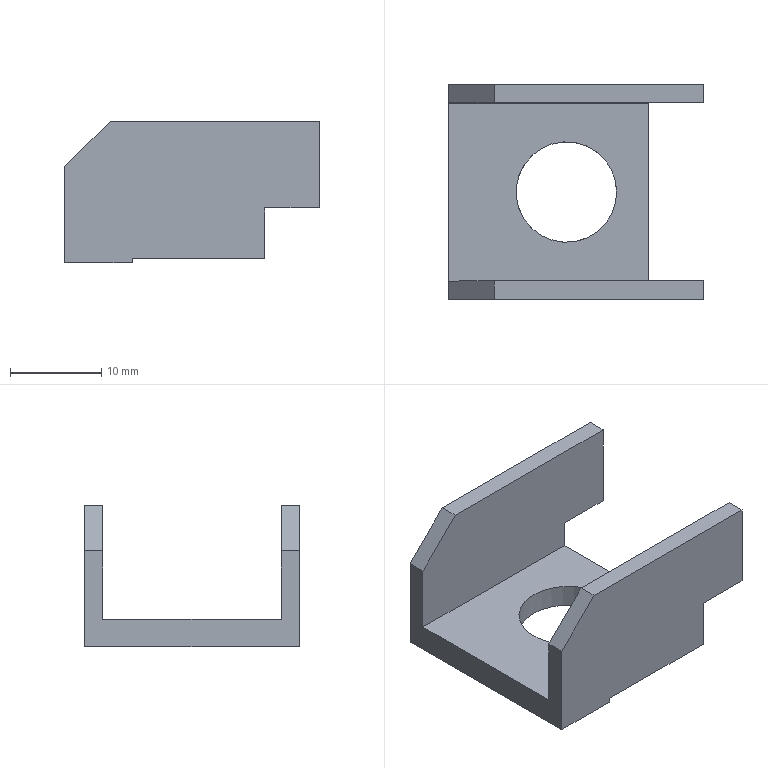Part | NX | features MAIN_BODY 2 | 1 solid | 19 faces | box 27.9 x 23.5 x 15.5 mm | volume 2409 mm3 | plane 18 | cylinder 1 | commonest cylinder face diameters 11 x1
STEP:
#1=CARTESIAN_POINT('',(961.102,239.333,238.));
#2=VERTEX_POINT('',#1);
#3=CARTESIAN_POINT('',(961.102,219.833,238.));
#4=VERTEX_POINT('',#3);
#5=CARTESIAN_POINT('',(961.102,241.333,238.));
#6=DIRECTION('',(0.,-1.,0.));
#7=VECTOR('',#6,1000.);
#8=LINE('',#5,#7);
#9=EDGE_CURVE('',#2,#4,#8,.T.);
#10=ORIENTED_EDGE('',*,*,#9,.T.);
#11=CARTESIAN_POINT('',(983.002,219.833,238.));
#12=VERTEX_POINT('',#11);
#13=CARTESIAN_POINT('',(973.552,219.833,238.));
#14=DIRECTION('',(-1.,0.,0.));
#15=VECTOR('',#14,1000.);
#16=LINE('',#13,#15);
#17=EDGE_CURVE('',#12,#4,#16,.T.);
#18=ORIENTED_EDGE('',*,*,#17,.F.);
#19=CARTESIAN_POINT('',(983.002,239.333,238.));
#20=VERTEX_POINT('',#19);
#21=CARTESIAN_POINT('',(983.002,241.333,238.));
#22=DIRECTION('',(0.,-1.,0.));
#23=VECTOR('',#22,1000.);
#24=LINE('',#21,#23);
#25=EDGE_CURVE('',#20,#12,#24,.T.);
#26=ORIENTED_EDGE('',*,*,#25,.F.);
#27=CARTESIAN_POINT('',(973.552,239.333,238.));
#28=DIRECTION('',(1.,0.,0.));
#29=VECTOR('',#28,1000.);
#30=LINE('',#27,#29);
#31=EDGE_CURVE('',#2,#20,#30,.T.);
#32=ORIENTED_EDGE('',*,*,#31,.F.);
#33=EDGE_LOOP('',(#10,#18,#26,#32));
#34=FACE_BOUND('',#33,.T.);
#35=CARTESIAN_POINT('',(979.502,229.583,238.));
#36=VERTEX_POINT('',#35);
#37=CARTESIAN_POINT('',(974.002,229.583,238.));
#38=DIRECTION('',(0.,0.,1.));
#39=DIRECTION('',(1.,0.,0.));
#40=AXIS2_PLACEMENT_3D('',#37,#38,#39);
#41=CIRCLE('',#40,5.5);
#42=EDGE_CURVE('',#36,#36,#41,.F.);
#43=ORIENTED_EDGE('',*,*,#42,.T.);
#44=EDGE_LOOP('',(#43));
#45=FACE_BOUND('',#44,.T.);
#46=CARTESIAN_POINT('',(973.552,229.583,238.));
#47=DIRECTION('',(0.,0.,-1.));
#48=DIRECTION('',(1.,0.,0.));
#49=AXIS2_PLACEMENT_3D('',#46,#47,#48);
#50=PLANE('',#49);
#51=ADVANCED_FACE('',(#34,#45),#50,.F.);
#52=CARTESIAN_POINT('',(968.502,241.333,235.5));
#53=VERTEX_POINT('',#52);
#54=CARTESIAN_POINT('',(968.502,229.583,235.5));
#55=VERTEX_POINT('',#54);
#56=CARTESIAN_POINT('',(968.502,241.333,235.5));
#57=DIRECTION('',(0.,-1.,0.));
#58=VECTOR('',#57,1000.);
#59=LINE('',#56,#58);
#60=EDGE_CURVE('',#53,#55,#59,.T.);
#61=ORIENTED_EDGE('',*,*,#60,.F.);
#62=CARTESIAN_POINT('',(983.002,241.333,235.5));
#63=VERTEX_POINT('',#62);
#64=CARTESIAN_POINT('',(983.002,241.333,235.5));
#65=DIRECTION('',(1.,0.,0.));
#66=VECTOR('',#65,1000.);
#67=LINE('',#64,#66);
#68=EDGE_CURVE('',#63,#53,#67,.F.);
#69=ORIENTED_EDGE('',*,*,#68,.F.);
#70=CARTESIAN_POINT('',(983.002,217.833,235.5));
#71=VERTEX_POINT('',#70);
#72=CARTESIAN_POINT('',(983.002,241.333,235.5));
#73=DIRECTION('',(0.,1.,0.));
#74=VECTOR('',#73,1000.);
#75=LINE('',#72,#74);
#76=EDGE_CURVE('',#71,#63,#75,.T.);
#77=ORIENTED_EDGE('',*,*,#76,.F.);
#78=CARTESIAN_POINT('',(968.502,217.833,235.5));
#79=VERTEX_POINT('',#78);
#80=CARTESIAN_POINT('',(983.002,217.833,235.5));
#81=DIRECTION('',(1.,0.,0.));
#82=VECTOR('',#81,1000.);
#83=LINE('',#80,#82);
#84=EDGE_CURVE('',#71,#79,#83,.F.);
#85=ORIENTED_EDGE('',*,*,#84,.T.);
#86=CARTESIAN_POINT('',(968.502,241.333,235.5));
#87=DIRECTION('',(0.,-1.,0.));
#88=VECTOR('',#87,1000.);
#89=LINE('',#86,#88);
#90=EDGE_CURVE('',#55,#79,#89,.T.);
#91=ORIENTED_EDGE('',*,*,#90,.F.);
#92=CARTESIAN_POINT('',(974.002,229.583,235.5));
#93=DIRECTION('',(0.,0.,1.));
#94=DIRECTION('',(1.,0.,0.));
#95=AXIS2_PLACEMENT_3D('',#92,#93,#94);
#96=CIRCLE('',#95,5.5);
#97=EDGE_CURVE('',#55,#55,#96,.F.);
#98=ORIENTED_EDGE('',*,*,#97,.F.);
#99=EDGE_LOOP('',(#61,#69,#77,#85,#91,#98));
#100=FACE_BOUND('',#99,.T.);
#101=CARTESIAN_POINT('',(983.002,241.333,235.5));
#102=DIRECTION('',(0.,0.,-1.));
#103=DIRECTION('',(0.,-1.,0.));
#104=AXIS2_PLACEMENT_3D('',#101,#102,#103);
#105=PLANE('',#104);
#106=ADVANCED_FACE('',(#100),#105,.T.);
#107=CARTESIAN_POINT('',(961.102,217.833,235.));
#108=VERTEX_POINT('',#107);
#109=CARTESIAN_POINT('',(968.502,217.833,235.));
#110=VERTEX_POINT('',#109);
#111=CARTESIAN_POINT('',(961.102,217.833,235.));
#112=DIRECTION('',(1.,0.,0.));
#113=VECTOR('',#112,1000.);
#114=LINE('',#111,#113);
#115=EDGE_CURVE('',#108,#110,#114,.T.);
#116=ORIENTED_EDGE('',*,*,#115,.F.);
#117=CARTESIAN_POINT('',(961.102,241.333,235.));
#118=VERTEX_POINT('',#117);
#119=CARTESIAN_POINT('',(961.102,241.333,235.));
#120=DIRECTION('',(0.,-1.,0.));
#121=VECTOR('',#120,1000.);
#122=LINE('',#119,#121);
#123=EDGE_CURVE('',#118,#108,#122,.T.);
#124=ORIENTED_EDGE('',*,*,#123,.F.);
#125=CARTESIAN_POINT('',(968.502,241.333,235.));
#126=VERTEX_POINT('',#125);
#127=CARTESIAN_POINT('',(989.002,241.333,235.));
#128=DIRECTION('',(-1.,0.,0.));
#129=VECTOR('',#128,1000.);
#130=LINE('',#127,#129);
#131=EDGE_CURVE('',#126,#118,#130,.T.);
#132=ORIENTED_EDGE('',*,*,#131,.F.);
#133=CARTESIAN_POINT('',(968.502,241.333,235.));
#134=DIRECTION('',(0.,-1.,0.));
#135=VECTOR('',#134,1000.);
#136=LINE('',#133,#135);
#137=EDGE_CURVE('',#126,#110,#136,.T.);
#138=ORIENTED_EDGE('',*,*,#137,.T.);
#139=EDGE_LOOP('',(#116,#124,#132,#138));
#140=FACE_BOUND('',#139,.T.);
#141=CARTESIAN_POINT('',(973.552,229.583,235.));
#142=DIRECTION('',(0.,0.,-1.));
#143=DIRECTION('',(1.,0.,0.));
#144=AXIS2_PLACEMENT_3D('',#141,#142,#143);
#145=PLANE('',#144);
#146=ADVANCED_FACE('',(#140),#145,.T.);
#147=ORIENTED_EDGE('',*,*,#76,.T.);
#148=CARTESIAN_POINT('',(983.002,241.333,241.));
#149=VERTEX_POINT('',#148);
#150=CARTESIAN_POINT('',(983.002,241.333,235.));
#151=DIRECTION('',(0.,0.,1.));
#152=VECTOR('',#151,1000.);
#153=LINE('',#150,#152);
#154=EDGE_CURVE('',#63,#149,#153,.T.);
#155=ORIENTED_EDGE('',*,*,#154,.T.);
#156=CARTESIAN_POINT('',(983.002,239.333,241.));
#157=VERTEX_POINT('',#156);
#158=CARTESIAN_POINT('',(983.002,241.333,241.));
#159=DIRECTION('',(0.,-1.,0.));
#160=VECTOR('',#159,1000.);
#161=LINE('',#158,#160);
#162=EDGE_CURVE('',#149,#157,#161,.T.);
#163=ORIENTED_EDGE('',*,*,#162,.T.);
#164=CARTESIAN_POINT('',(983.002,239.333,235.));
#165=DIRECTION('',(0.,0.,-1.));
#166=VECTOR('',#165,1000.);
#167=LINE('',#164,#166);
#168=EDGE_CURVE('',#157,#20,#167,.T.);
#169=ORIENTED_EDGE('',*,*,#168,.T.);
#170=ORIENTED_EDGE('',*,*,#25,.T.);
#171=CARTESIAN_POINT('',(983.002,219.833,241.));
#172=VERTEX_POINT('',#171);
#173=CARTESIAN_POINT('',(983.002,219.833,235.));
#174=DIRECTION('',(0.,0.,1.));
#175=VECTOR('',#174,1000.);
#176=LINE('',#173,#175);
#177=EDGE_CURVE('',#12,#172,#176,.T.);
#178=ORIENTED_EDGE('',*,*,#177,.T.);
#179=CARTESIAN_POINT('',(983.002,217.833,241.));
#180=VERTEX_POINT('',#179);
#181=CARTESIAN_POINT('',(983.002,241.333,241.));
#182=DIRECTION('',(0.,-1.,0.));
#183=VECTOR('',#182,1000.);
#184=LINE('',#181,#183);
#185=EDGE_CURVE('',#172,#180,#184,.T.);
#186=ORIENTED_EDGE('',*,*,#185,.T.);
#187=CARTESIAN_POINT('',(983.002,217.833,235.));
#188=DIRECTION('',(0.,0.,1.));
#189=VECTOR('',#188,1000.);
#190=LINE('',#187,#189);
#191=EDGE_CURVE('',#71,#180,#190,.T.);
#192=ORIENTED_EDGE('',*,*,#191,.F.);
#193=EDGE_LOOP('',(#147,#155,#163,#169,#170,#178,#186,#192));
#194=FACE_BOUND('',#193,.T.);
#195=CARTESIAN_POINT('',(983.002,241.333,238.));
#196=DIRECTION('',(-1.,0.,0.));
#197=DIRECTION('',(0.,1.,0.));
#198=AXIS2_PLACEMENT_3D('',#195,#196,#197);
#199=PLANE('',#198);
#200=ADVANCED_FACE('',(#194),#199,.F.);
#201=CARTESIAN_POINT('',(989.002,241.333,250.5));
#202=VERTEX_POINT('',#201);
#203=CARTESIAN_POINT('',(966.102,241.333,250.5));
#204=VERTEX_POINT('',#203);
#205=CARTESIAN_POINT('',(989.002,241.333,250.5));
#206=DIRECTION('',(-1.,0.,0.));
#207=VECTOR('',#206,1000.);
#208=LINE('',#205,#207);
#209=EDGE_CURVE('',#202,#204,#208,.T.);
#210=ORIENTED_EDGE('',*,*,#209,.F.);
#211=CARTESIAN_POINT('',(989.002,241.333,241.));
#212=VERTEX_POINT('',#211);
#213=CARTESIAN_POINT('',(989.002,241.333,235.));
#214=DIRECTION('',(0.,0.,1.));
#215=VECTOR('',#214,1000.);
#216=LINE('',#213,#215);
#217=EDGE_CURVE('',#212,#202,#216,.T.);
#218=ORIENTED_EDGE('',*,*,#217,.F.);
#219=CARTESIAN_POINT('',(983.002,241.333,241.));
#220=DIRECTION('',(1.,0.,0.));
#221=VECTOR('',#220,1000.);
#222=LINE('',#219,#221);
#223=EDGE_CURVE('',#149,#212,#222,.T.);
#224=ORIENTED_EDGE('',*,*,#223,.F.);
#225=ORIENTED_EDGE('',*,*,#154,.F.);
#226=ORIENTED_EDGE('',*,*,#68,.T.);
#227=CARTESIAN_POINT('',(968.502,241.333,235.));
#228=DIRECTION('',(0.,0.,1.));
#229=VECTOR('',#228,1000.);
#230=LINE('',#227,#229);
#231=EDGE_CURVE('',#126,#53,#230,.T.);
#232=ORIENTED_EDGE('',*,*,#231,.F.);
#233=ORIENTED_EDGE('',*,*,#131,.T.);
#234=CARTESIAN_POINT('',(961.102,241.333,245.5));
#235=VERTEX_POINT('',#234);
#236=CARTESIAN_POINT('',(961.102,241.333,238.));
#237=DIRECTION('',(0.,0.,-1.));
#238=VECTOR('',#237,1000.);
#239=LINE('',#236,#238);
#240=EDGE_CURVE('',#235,#118,#239,.T.);
#241=ORIENTED_EDGE('',*,*,#240,.F.);
#242=CARTESIAN_POINT('',(971.302,241.333,255.7));
#243=DIRECTION('',(-0.7071,0.,-0.7071));
#244=VECTOR('',#243,1000.);
#245=LINE('',#242,#244);
#246=EDGE_CURVE('',#204,#235,#245,.T.);
#247=ORIENTED_EDGE('',*,*,#246,.F.);
#248=EDGE_LOOP('',(#210,#218,#224,#225,#226,#232,#233,#241,#247));
#249=FACE_BOUND('',#248,.T.);
#250=CARTESIAN_POINT('',(989.002,241.333,238.));
#251=DIRECTION('',(0.,1.,0.));
#252=DIRECTION('',(0.,0.,1.));
#253=AXIS2_PLACEMENT_3D('',#250,#251,#252);
#254=PLANE('',#253);
#255=ADVANCED_FACE('',(#249),#254,.T.);
#256=CARTESIAN_POINT('',(961.102,217.833,245.5));
#257=VERTEX_POINT('',#256);
#258=CARTESIAN_POINT('',(961.102,217.833,238.));
#259=DIRECTION('',(0.,0.,-1.));
#260=VECTOR('',#259,1000.);
#261=LINE('',#258,#260);
#262=EDGE_CURVE('',#257,#108,#261,.T.);
#263=ORIENTED_EDGE('',*,*,#262,.T.);
#264=ORIENTED_EDGE('',*,*,#115,.T.);
#265=CARTESIAN_POINT('',(968.502,217.833,235.));
#266=DIRECTION('',(0.,0.,1.));
#267=VECTOR('',#266,1000.);
#268=LINE('',#265,#267);
#269=EDGE_CURVE('',#110,#79,#268,.T.);
#270=ORIENTED_EDGE('',*,*,#269,.T.);
#271=ORIENTED_EDGE('',*,*,#84,.F.);
#272=ORIENTED_EDGE('',*,*,#191,.T.);
#273=CARTESIAN_POINT('',(989.002,217.833,241.));
#274=VERTEX_POINT('',#273);
#275=CARTESIAN_POINT('',(983.002,217.833,241.));
#276=DIRECTION('',(1.,0.,0.));
#277=VECTOR('',#276,1000.);
#278=LINE('',#275,#277);
#279=EDGE_CURVE('',#180,#274,#278,.T.);
#280=ORIENTED_EDGE('',*,*,#279,.T.);
#281=CARTESIAN_POINT('',(989.002,217.833,250.5));
#282=VERTEX_POINT('',#281);
#283=CARTESIAN_POINT('',(989.002,217.833,235.));
#284=DIRECTION('',(0.,0.,1.));
#285=VECTOR('',#284,1000.);
#286=LINE('',#283,#285);
#287=EDGE_CURVE('',#274,#282,#286,.T.);
#288=ORIENTED_EDGE('',*,*,#287,.T.);
#289=CARTESIAN_POINT('',(966.102,217.833,250.5));
#290=VERTEX_POINT('',#289);
#291=CARTESIAN_POINT('',(961.102,217.833,250.5));
#292=DIRECTION('',(1.,0.,0.));
#293=VECTOR('',#292,1000.);
#294=LINE('',#291,#293);
#295=EDGE_CURVE('',#290,#282,#294,.T.);
#296=ORIENTED_EDGE('',*,*,#295,.F.);
#297=CARTESIAN_POINT('',(957.352,217.833,241.75));
#298=DIRECTION('',(0.7071,0.,0.7071));
#299=VECTOR('',#298,1000.);
#300=LINE('',#297,#299);
#301=EDGE_CURVE('',#257,#290,#300,.T.);
#302=ORIENTED_EDGE('',*,*,#301,.F.);
#303=EDGE_LOOP('',(#263,#264,#270,#271,#272,#280,#288,#296,#302));
#304=FACE_BOUND('',#303,.T.);
#305=CARTESIAN_POINT('',(961.102,217.833,238.));
#306=DIRECTION('',(0.,-1.,0.));
#307=DIRECTION('',(-1.,0.,0.));
#308=AXIS2_PLACEMENT_3D('',#305,#306,#307);
#309=PLANE('',#308);
#310=ADVANCED_FACE('',(#304),#309,.T.);
#311=CARTESIAN_POINT('',(961.102,219.833,245.5));
#312=VERTEX_POINT('',#311);
#313=CARTESIAN_POINT('',(961.102,219.833,235.));
#314=DIRECTION('',(0.,0.,1.));
#315=VECTOR('',#314,1000.);
#316=LINE('',#313,#315);
#317=EDGE_CURVE('',#4,#312,#316,.T.);
#318=ORIENTED_EDGE('',*,*,#317,.F.);
#319=ORIENTED_EDGE('',*,*,#9,.F.);
#320=CARTESIAN_POINT('',(961.102,239.333,245.5));
#321=VERTEX_POINT('',#320);
#322=CARTESIAN_POINT('',(961.102,239.333,235.));
#323=DIRECTION('',(0.,0.,-1.));
#324=VECTOR('',#323,1000.);
#325=LINE('',#322,#324);
#326=EDGE_CURVE('',#2,#321,#325,.F.);
#327=ORIENTED_EDGE('',*,*,#326,.T.);
#328=CARTESIAN_POINT('',(961.102,241.333,245.5));
#329=DIRECTION('',(0.,-1.,0.));
#330=VECTOR('',#329,1000.);
#331=LINE('',#328,#330);
#332=EDGE_CURVE('',#235,#321,#331,.T.);
#333=ORIENTED_EDGE('',*,*,#332,.F.);
#334=ORIENTED_EDGE('',*,*,#240,.T.);
#335=ORIENTED_EDGE('',*,*,#123,.T.);
#336=ORIENTED_EDGE('',*,*,#262,.F.);
#337=CARTESIAN_POINT('',(961.102,241.333,245.5));
#338=DIRECTION('',(0.,-1.,0.));
#339=VECTOR('',#338,1000.);
#340=LINE('',#337,#339);
#341=EDGE_CURVE('',#312,#257,#340,.T.);
#342=ORIENTED_EDGE('',*,*,#341,.F.);
#343=EDGE_LOOP('',(#318,#319,#327,#333,#334,#335,#336,#342));
#344=FACE_BOUND('',#343,.T.);
#345=CARTESIAN_POINT('',(961.102,241.333,238.));
#346=DIRECTION('',(-1.,0.,0.));
#347=DIRECTION('',(0.,0.,-1.));
#348=AXIS2_PLACEMENT_3D('',#345,#346,#347);
#349=PLANE('',#348);
#350=ADVANCED_FACE('',(#344),#349,.T.);
#351=CARTESIAN_POINT('',(966.102,219.833,250.5));
#352=VERTEX_POINT('',#351);
#353=CARTESIAN_POINT('',(989.002,219.833,250.5));
#354=VERTEX_POINT('',#353);
#355=CARTESIAN_POINT('',(961.102,219.833,250.5));
#356=DIRECTION('',(1.,0.,0.));
#357=VECTOR('',#356,1000.);
#358=LINE('',#355,#357);
#359=EDGE_CURVE('',#352,#354,#358,.T.);
#360=ORIENTED_EDGE('',*,*,#359,.T.);
#361=CARTESIAN_POINT('',(989.002,219.833,241.));
#362=VERTEX_POINT('',#361);
#363=CARTESIAN_POINT('',(989.002,219.833,235.));
#364=DIRECTION('',(0.,0.,1.));
#365=VECTOR('',#364,1000.);
#366=LINE('',#363,#365);
#367=EDGE_CURVE('',#362,#354,#366,.T.);
#368=ORIENTED_EDGE('',*,*,#367,.F.);
#369=CARTESIAN_POINT('',(961.102,219.833,241.));
#370=DIRECTION('',(1.,0.,0.));
#371=VECTOR('',#370,1000.);
#372=LINE('',#369,#371);
#373=EDGE_CURVE('',#362,#172,#372,.F.);
#374=ORIENTED_EDGE('',*,*,#373,.T.);
#375=ORIENTED_EDGE('',*,*,#177,.F.);
#376=ORIENTED_EDGE('',*,*,#17,.T.);
#377=ORIENTED_EDGE('',*,*,#317,.T.);
#378=CARTESIAN_POINT('',(955.852,219.833,240.25));
#379=DIRECTION('',(-0.7071,0.,-0.7071));
#380=VECTOR('',#379,1000.);
#381=LINE('',#378,#380);
#382=EDGE_CURVE('',#352,#312,#381,.T.);
#383=ORIENTED_EDGE('',*,*,#382,.F.);
#384=EDGE_LOOP('',(#360,#368,#374,#375,#376,#377,#383));
#385=FACE_BOUND('',#384,.T.);
#386=CARTESIAN_POINT('',(961.102,219.833,235.));
#387=DIRECTION('',(0.,1.,0.));
#388=DIRECTION('',(1.,0.,0.));
#389=AXIS2_PLACEMENT_3D('',#386,#387,#388);
#390=PLANE('',#389);
#391=ADVANCED_FACE('',(#385),#390,.T.);
#392=CARTESIAN_POINT('',(989.002,217.833,241.));
#393=DIRECTION('',(0.,-1.,0.));
#394=VECTOR('',#393,1000.);
#395=LINE('',#392,#394);
#396=EDGE_CURVE('',#274,#362,#395,.F.);
#397=ORIENTED_EDGE('',*,*,#396,.T.);
#398=ORIENTED_EDGE('',*,*,#367,.T.);
#399=CARTESIAN_POINT('',(989.002,217.833,250.5));
#400=DIRECTION('',(0.,1.,0.));
#401=VECTOR('',#400,1000.);
#402=LINE('',#399,#401);
#403=EDGE_CURVE('',#282,#354,#402,.T.);
#404=ORIENTED_EDGE('',*,*,#403,.F.);
#405=ORIENTED_EDGE('',*,*,#287,.F.);
#406=EDGE_LOOP('',(#397,#398,#404,#405));
#407=FACE_BOUND('',#406,.T.);
#408=CARTESIAN_POINT('',(989.002,217.833,235.));
#409=DIRECTION('',(1.,0.,0.));
#410=DIRECTION('',(0.,0.,1.));
#411=AXIS2_PLACEMENT_3D('',#408,#409,#410);
#412=PLANE('',#411);
#413=ADVANCED_FACE('',(#407),#412,.T.);
#414=ORIENTED_EDGE('',*,*,#295,.T.);
#415=ORIENTED_EDGE('',*,*,#403,.T.);
#416=ORIENTED_EDGE('',*,*,#359,.F.);
#417=CARTESIAN_POINT('',(966.102,217.833,250.5));
#418=DIRECTION('',(0.,-1.,0.));
#419=VECTOR('',#418,1000.);
#420=LINE('',#417,#419);
#421=EDGE_CURVE('',#290,#352,#420,.F.);
#422=ORIENTED_EDGE('',*,*,#421,.F.);
#423=EDGE_LOOP('',(#414,#415,#416,#422));
#424=FACE_BOUND('',#423,.T.);
#425=CARTESIAN_POINT('',(961.102,217.833,250.5));
#426=DIRECTION('',(0.,0.,-1.));
#427=DIRECTION('',(1.,0.,0.));
#428=AXIS2_PLACEMENT_3D('',#425,#426,#427);
#429=PLANE('',#428);
#430=ADVANCED_FACE('',(#424),#429,.F.);
#431=ORIENTED_EDGE('',*,*,#326,.F.);
#432=ORIENTED_EDGE('',*,*,#31,.T.);
#433=ORIENTED_EDGE('',*,*,#168,.F.);
#434=CARTESIAN_POINT('',(989.002,239.333,241.));
#435=VERTEX_POINT('',#434);
#436=CARTESIAN_POINT('',(989.002,239.333,241.));
#437=DIRECTION('',(-1.,0.,0.));
#438=VECTOR('',#437,1000.);
#439=LINE('',#436,#438);
#440=EDGE_CURVE('',#157,#435,#439,.F.);
#441=ORIENTED_EDGE('',*,*,#440,.T.);
#442=CARTESIAN_POINT('',(989.002,239.333,250.5));
#443=VERTEX_POINT('',#442);
#444=CARTESIAN_POINT('',(989.002,239.333,235.));
#445=DIRECTION('',(0.,0.,-1.));
#446=VECTOR('',#445,1000.);
#447=LINE('',#444,#446);
#448=EDGE_CURVE('',#435,#443,#447,.F.);
#449=ORIENTED_EDGE('',*,*,#448,.T.);
#450=CARTESIAN_POINT('',(966.102,239.333,250.5));
#451=VERTEX_POINT('',#450);
#452=CARTESIAN_POINT('',(989.002,239.333,250.5));
#453=DIRECTION('',(-1.,0.,0.));
#454=VECTOR('',#453,1000.);
#455=LINE('',#452,#454);
#456=EDGE_CURVE('',#443,#451,#455,.T.);
#457=ORIENTED_EDGE('',*,*,#456,.T.);
#458=CARTESIAN_POINT('',(969.802,239.333,254.2));
#459=DIRECTION('',(0.7071,0.,0.7071));
#460=VECTOR('',#459,1000.);
#461=LINE('',#458,#460);
#462=EDGE_CURVE('',#321,#451,#461,.T.);
#463=ORIENTED_EDGE('',*,*,#462,.F.);
#464=EDGE_LOOP('',(#431,#432,#433,#441,#449,#457,#463));
#465=FACE_BOUND('',#464,.T.);
#466=CARTESIAN_POINT('',(989.002,239.333,235.));
#467=DIRECTION('',(0.,-1.,0.));
#468=DIRECTION('',(0.,0.,-1.));
#469=AXIS2_PLACEMENT_3D('',#466,#467,#468);
#470=PLANE('',#469);
#471=ADVANCED_FACE('',(#465),#470,.T.);
#472=ORIENTED_EDGE('',*,*,#456,.F.);
#473=CARTESIAN_POINT('',(989.002,241.333,250.5));
#474=DIRECTION('',(0.,-1.,0.));
#475=VECTOR('',#474,1000.);
#476=LINE('',#473,#475);
#477=EDGE_CURVE('',#202,#443,#476,.T.);
#478=ORIENTED_EDGE('',*,*,#477,.F.);
#479=ORIENTED_EDGE('',*,*,#209,.T.);
#480=CARTESIAN_POINT('',(966.102,241.333,250.5));
#481=DIRECTION('',(0.,-1.,0.));
#482=VECTOR('',#481,1000.);
#483=LINE('',#480,#482);
#484=EDGE_CURVE('',#451,#204,#483,.F.);
#485=ORIENTED_EDGE('',*,*,#484,.F.);
#486=EDGE_LOOP('',(#472,#478,#479,#485));
#487=FACE_BOUND('',#486,.T.);
#488=CARTESIAN_POINT('',(989.002,241.333,250.5));
#489=DIRECTION('',(0.,0.,-1.));
#490=DIRECTION('',(-1.,0.,0.));
#491=AXIS2_PLACEMENT_3D('',#488,#489,#490);
#492=PLANE('',#491);
#493=ADVANCED_FACE('',(#487),#492,.F.);
#494=CARTESIAN_POINT('',(989.002,241.333,241.));
#495=DIRECTION('',(0.,1.,0.));
#496=VECTOR('',#495,1000.);
#497=LINE('',#494,#496);
#498=EDGE_CURVE('',#435,#212,#497,.T.);
#499=ORIENTED_EDGE('',*,*,#498,.T.);
#500=ORIENTED_EDGE('',*,*,#217,.T.);
#501=ORIENTED_EDGE('',*,*,#477,.T.);
#502=ORIENTED_EDGE('',*,*,#448,.F.);
#503=EDGE_LOOP('',(#499,#500,#501,#502));
#504=FACE_BOUND('',#503,.T.);
#505=CARTESIAN_POINT('',(989.002,241.333,235.));
#506=DIRECTION('',(-1.,0.,0.));
#507=DIRECTION('',(0.,0.,1.));
#508=AXIS2_PLACEMENT_3D('',#505,#506,#507);
#509=PLANE('',#508);
#510=ADVANCED_FACE('',(#504),#509,.F.);
#511=ORIENTED_EDGE('',*,*,#440,.F.);
#512=ORIENTED_EDGE('',*,*,#162,.F.);
#513=ORIENTED_EDGE('',*,*,#223,.T.);
#514=ORIENTED_EDGE('',*,*,#498,.F.);
#515=EDGE_LOOP('',(#511,#512,#513,#514));
#516=FACE_BOUND('',#515,.T.);
#517=CARTESIAN_POINT('',(983.002,241.333,241.));
#518=DIRECTION('',(0.,0.,-1.));
#519=DIRECTION('',(0.,-1.,0.));
#520=AXIS2_PLACEMENT_3D('',#517,#518,#519);
#521=PLANE('',#520);
#522=ADVANCED_FACE('',(#516),#521,.T.);
#523=ORIENTED_EDGE('',*,*,#373,.F.);
#524=ORIENTED_EDGE('',*,*,#396,.F.);
#525=ORIENTED_EDGE('',*,*,#279,.F.);
#526=ORIENTED_EDGE('',*,*,#185,.F.);
#527=EDGE_LOOP('',(#523,#524,#525,#526));
#528=FACE_BOUND('',#527,.T.);
#529=CARTESIAN_POINT('',(983.002,241.333,241.));
#530=DIRECTION('',(0.,0.,-1.));
#531=DIRECTION('',(0.,-1.,0.));
#532=AXIS2_PLACEMENT_3D('',#529,#530,#531);
#533=PLANE('',#532);
#534=ADVANCED_FACE('',(#528),#533,.T.);
#535=ORIENTED_EDGE('',*,*,#90,.T.);
#536=ORIENTED_EDGE('',*,*,#269,.F.);
#537=ORIENTED_EDGE('',*,*,#137,.F.);
#538=ORIENTED_EDGE('',*,*,#231,.T.);
#539=ORIENTED_EDGE('',*,*,#60,.T.);
#540=EDGE_LOOP('',(#535,#536,#537,#538,#539));
#541=FACE_BOUND('',#540,.T.);
#542=CARTESIAN_POINT('',(968.502,241.333,235.));
#543=DIRECTION('',(1.,0.,0.));
#544=DIRECTION('',(0.,-1.,0.));
#545=AXIS2_PLACEMENT_3D('',#542,#543,#544);
#546=PLANE('',#545);
#547=ADVANCED_FACE('',(#541),#546,.T.);
#548=ORIENTED_EDGE('',*,*,#97,.T.);
#549=EDGE_LOOP('',(#548));
#550=FACE_BOUND('',#549,.T.);
#551=ORIENTED_EDGE('',*,*,#42,.F.);
#552=EDGE_LOOP('',(#551));
#553=FACE_BOUND('',#552,.T.);
#554=CARTESIAN_POINT('',(974.002,229.583,285.));
#555=DIRECTION('',(0.,0.,-1.));
#556=DIRECTION('',(1.,0.,0.));
#557=AXIS2_PLACEMENT_3D('',#554,#555,#556);
#558=CYLINDRICAL_SURFACE('',#557,5.5);
#559=ADVANCED_FACE('',(#550,#553),#558,.F.);
#560=ORIENTED_EDGE('',*,*,#301,.T.);
#561=ORIENTED_EDGE('',*,*,#421,.T.);
#562=ORIENTED_EDGE('',*,*,#382,.T.);
#563=ORIENTED_EDGE('',*,*,#341,.T.);
#564=EDGE_LOOP('',(#560,#561,#562,#563));
#565=FACE_BOUND('',#564,.T.);
#566=CARTESIAN_POINT('',(966.102,217.833,250.5));
#567=DIRECTION('',(-0.7071,0.,0.7071));
#568=DIRECTION('',(-0.7071,0.,-0.7071));
#569=AXIS2_PLACEMENT_3D('',#566,#567,#568);
#570=PLANE('',#569);
#571=ADVANCED_FACE('',(#565),#570,.T.);
#572=ORIENTED_EDGE('',*,*,#246,.T.);
#573=ORIENTED_EDGE('',*,*,#332,.T.);
#574=ORIENTED_EDGE('',*,*,#462,.T.);
#575=ORIENTED_EDGE('',*,*,#484,.T.);
#576=EDGE_LOOP('',(#572,#573,#574,#575));
#577=FACE_BOUND('',#576,.T.);
#578=CARTESIAN_POINT('',(961.102,241.333,245.5));
#579=DIRECTION('',(-0.7071,0.,0.7071));
#580=DIRECTION('',(-0.7071,0.,-0.7071));
#581=AXIS2_PLACEMENT_3D('',#578,#579,#580);
#582=PLANE('',#581);
#583=ADVANCED_FACE('',(#577),#582,.T.);
#584=CLOSED_SHELL('',(#51,#106,#146,#200,#255,#310,#350,#391,#413,#430,#471,#493,#510,#522,#534,#547,#559,#571,#583));
#585=MANIFOLD_SOLID_BREP('',#584);
#586=(LENGTH_UNIT()NAMED_UNIT(*)SI_UNIT(.MILLI.,.METRE.));
#587=UNCERTAINTY_MEASURE_WITH_UNIT(LENGTH_MEASURE(0.00001),#586,'','');
#588=(NAMED_UNIT(*)PLANE_ANGLE_UNIT()SI_UNIT($,.RADIAN.));
#589=(NAMED_UNIT(*)SI_UNIT($,.STERADIAN.)SOLID_ANGLE_UNIT());
#590=(GEOMETRIC_REPRESENTATION_CONTEXT(3)GLOBAL_UNCERTAINTY_ASSIGNED_CONTEXT((#587))GLOBAL_UNIT_ASSIGNED_CONTEXT((#586,#588,#589))REPRESENTATION_CONTEXT('',''));
#591=ADVANCED_BREP_SHAPE_REPRESENTATION('',(#585),#590);